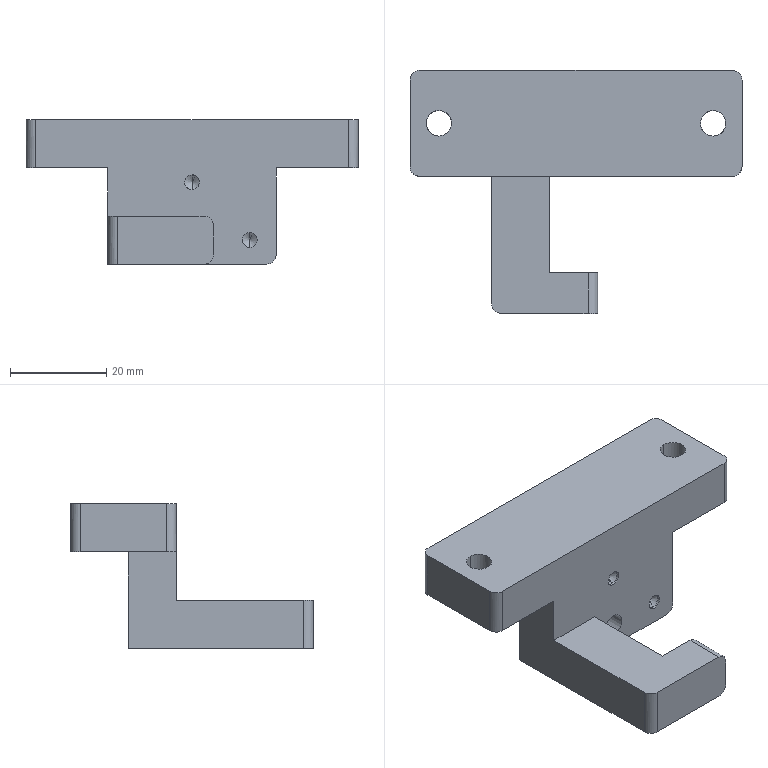NC program | NX | posted with a generic post | part box 69 x 50.5 x 30 mm
Lines 1 to 1585 of 2489:
N10 G17 G21 G94 G90
(FLOOR_WALL_COPY , TOOL : D80)
N12 T19 M6
N14 G54
N16 G17 G0 G90 X77.5 Y0. B0. C0. S6500 M3
N18 G43 Z30. H19
N20 Z7.
N22 G94 G1 Z4. F1500.
N24 X74.5
N26 X-74.5
N28 X-77.5
N30 Z7.
N32 G0 Z30.
N34 X77.5
N36 Z6.
N38 G1 Z3.
N40 X74.5
N42 X-74.5
N44 X-77.5
N46 Z6.
N48 G0 Z30.
N50 X77.5
N52 Z5.
N54 G1 Z2.
N56 X74.5
N58 X-74.5
N60 X-77.5
N62 Z5.
N64 G0 Z30.
N66 X77.5
N68 Z4.
N70 G1 Z1.
N72 X74.5
N74 X-74.5
N76 X-77.5
N78 Z4.
N80 G0 Z30.
N82 X77.5
N84 Z3.
N86 G1 Z0.
N88 X74.5
N90 X-74.5
N92 X-77.5
N94 Z3.
N96 G0 Z30.
N98 M5
(FLOOR_WALL_1_COPY_1 , TOOL : D10)
N100 T15 M6
N102 G54
N104 G17 G0 G90 X41. Y-12.807 B0. C0. S9500 M3
N106 G43 Z30. H15
N108 Z0.505
N110 G94 G1 Z-0.995 F3500.
N112 X40. Y-13.384
N114 G3 X39.5 Y-14.25 R1.
N116 G1 Y-23.479
N118 X39.403 Y-24.541
N120 X39.028 Y-25.845
N122 X38.378 Y-27.099
N124 X37.469 Y-28.219
N126 X36.349 Y-29.128
N128 X35.095 Y-29.778
N130 X33.791 Y-30.153
N132 X32.729 Y-30.25
N134 X-32.751
N136 X-33.878 Y-30.137
N138 X-35.185 Y-29.738
N140 X-36.392 Y-29.097
N142 X-37.468 Y-28.218
N144 X-38.347 Y-27.142
N146 X-38.988 Y-25.935
N148 X-39.387 Y-24.628
N150 X-39.5 Y-23.501
N152 Y-5.021
N154 X-39.403 Y-3.959
N156 X-39.028 Y-2.655
N158 X-38.378 Y-1.401
N160 X-37.469 Y-0.281
N162 X-36.349 Y0.628
N164 X-35.095 Y1.278
N166 X-33.791 Y1.653
N168 X-32.729 Y1.75
N170 X-22.6
N172 Y-18.35
N174 X-27.599 Y-23.25
N176 X-32.4
N178 X-32.491 Y-23.241
N180 X-32.492 Y-5.258
N182 X-32.408 Y-5.25
N184 X-29.6
N186 Y-18.35
N188 G3 X-27.599 Y-23.25 R7.
N190 G1 X-22.6 Y-18.35
N192 X22.6
N194 Y1.75
N196 X32.729
N198 X33.791 Y1.653
N200 X35.095 Y1.278
N202 X36.349 Y0.628
N204 X37.469 Y-0.281
N206 X38.378 Y-1.401
N208 X39.028 Y-2.655
N210 X39.403 Y-3.959
N212 X39.5 Y-5.021
N214 Y-14.25
N216 X32.5
N218 Y-23.158
N220 X32.492 Y-23.242
N222 X32.408 Y-23.25
N224 X27.599
N226 X22.6 Y-23.35
N228 X-22.6
N230 G2 X-23.016 Y-25.25 R5.
N232 G1 X23.016
N234 G2 X22.6 Y-23.35 R5.
N236 G1 X27.599 Y-23.25
N238 G3 X29.6 Y-18.35 R7.
N240 G1 Y-5.25
N242 X32.408
N244 X32.492 Y-5.258
N246 X32.5 Y-5.342
N248 Y-14.25
N250 G3 X33. Y-15.116 R1.
N252 G1 Z0.505
N254 G0 X41. Y-12.807 Z-0.49
N256 G1 Z-1.99
N258 X40. Y-13.384
N260 G3 X39.5 Y-14.25 R1.
N262 G1 Y-23.479
N264 X39.403 Y-24.541
N266 X39.028 Y-25.845
N268 X38.378 Y-27.099
N270 X37.469 Y-28.219
N272 X36.349 Y-29.128
N274 X35.095 Y-29.778
N276 X33.791 Y-30.153
N278 X32.729 Y-30.25
N280 X-32.751
N282 X-33.878 Y-30.137
N284 X-35.185 Y-29.738
N286 X-36.392 Y-29.097
N288 X-37.468 Y-28.218
N290 X-38.347 Y-27.142
N292 X-38.988 Y-25.935
N294 X-39.387 Y-24.628
N296 X-39.5 Y-23.501
N298 Y-5.021
N300 X-39.403 Y-3.959
N302 X-39.028 Y-2.655
N304 X-38.378 Y-1.401
N306 X-37.469 Y-0.281
N308 X-36.349 Y0.628
N310 X-35.095 Y1.278
N312 X-33.791 Y1.653
N314 X-32.729 Y1.75
N316 X-22.6
N318 Y-18.35
N320 X-27.599 Y-23.25
N322 X-32.4
N324 X-32.491 Y-23.241
N326 X-32.492 Y-5.258
N328 X-32.408 Y-5.25
N330 X-29.6
N332 Y-18.35
N334 G3 X-27.599 Y-23.25 R7.
N336 G1 X-22.6 Y-18.35
N338 X22.6
N340 Y1.75
N342 X32.729
N344 X33.791 Y1.653
N346 X35.095 Y1.278
N348 X36.349 Y0.628
N350 X37.469 Y-0.281
N352 X38.378 Y-1.401
N354 X39.028 Y-2.655
N356 X39.403 Y-3.959
N358 X39.5 Y-5.021
N360 Y-14.25
N362 X32.5
N364 Y-23.158
N366 X32.492 Y-23.242
N368 X32.408 Y-23.25
N370 X27.599
N372 X22.6 Y-23.35
N374 X-22.6
N376 G2 X-23.016 Y-25.25 R5.
N378 G1 X23.016
N380 G2 X22.6 Y-23.35 R5.
N382 G1 X27.599 Y-23.25
N384 G3 X29.6 Y-18.35 R7.
N386 G1 Y-5.25
N388 X32.408
N390 X32.492 Y-5.258
N392 X32.5 Y-5.342
N394 Y-14.25
N396 G3 X33. Y-15.116 R1.
N398 G1 Z-0.49
N400 G0 X41. Y-12.807 Z-1.485
N402 G1 Z-2.985
N404 X40. Y-13.384
N406 G3 X39.5 Y-14.25 R1.
N408 G1 Y-23.479
N410 X39.403 Y-24.541
N412 X39.028 Y-25.845
N414 X38.378 Y-27.099
N416 X37.469 Y-28.219
N418 X36.349 Y-29.128
N420 X35.095 Y-29.778
N422 X33.791 Y-30.153
N424 X32.729 Y-30.25
N426 X-32.751
N428 X-33.878 Y-30.137
N430 X-35.185 Y-29.738
N432 X-36.392 Y-29.097
N434 X-37.468 Y-28.218
N436 X-38.347 Y-27.142
N438 X-38.988 Y-25.935
N440 X-39.387 Y-24.628
N442 X-39.5 Y-23.501
N444 Y-5.021
N446 X-39.403 Y-3.959
N448 X-39.028 Y-2.655
N450 X-38.378 Y-1.401
N452 X-37.469 Y-0.281
N454 X-36.349 Y0.628
N456 X-35.095 Y1.278
N458 X-33.791 Y1.653
N460 X-32.729 Y1.75
N462 X-22.6
N464 Y-18.35
N466 X-27.599 Y-23.25
N468 X-32.4
N470 X-32.491 Y-23.241
N472 X-32.492 Y-5.258
N474 X-32.408 Y-5.25
N476 X-29.6
N478 Y-18.35
N480 G3 X-27.599 Y-23.25 R7.
N482 G1 X-22.6 Y-18.35
N484 X22.6
N486 Y1.75
N488 X32.729
N490 X33.791 Y1.653
N492 X35.095 Y1.278
N494 X36.349 Y0.628
N496 X37.469 Y-0.281
N498 X38.378 Y-1.401
N500 X39.028 Y-2.655
N502 X39.403 Y-3.959
N504 X39.5 Y-5.021
N506 Y-14.25
N508 X32.5
N510 Y-23.158
N512 X32.492 Y-23.242
N514 X32.408 Y-23.25
N516 X27.599
N518 X22.6 Y-23.35
N520 X-22.6
N522 G2 X-23.016 Y-25.25 R5.
N524 G1 X23.016
N526 G2 X22.6 Y-23.35 R5.
N528 G1 X27.599 Y-23.25
N530 G3 X29.6 Y-18.35 R7.
N532 G1 Y-5.25
N534 X32.408
N536 X32.492 Y-5.258
N538 X32.5 Y-5.342
N540 Y-14.25
N542 G3 X33. Y-15.116 R1.
N544 G1 Z-1.485
N546 G0 X41. Y-12.807 Z-2.48
N548 G1 Z-3.98
N550 X40. Y-13.384
N552 G3 X39.5 Y-14.25 R1.
N554 G1 Y-23.479
N556 X39.403 Y-24.541
N558 X39.028 Y-25.845
N560 X38.378 Y-27.099
N562 X37.469 Y-28.219
N564 X36.349 Y-29.128
N566 X35.095 Y-29.778
N568 X33.791 Y-30.153
N570 X32.729 Y-30.25
N572 X-32.751
N574 X-33.878 Y-30.137
N576 X-35.185 Y-29.738
N578 X-36.392 Y-29.097
N580 X-37.468 Y-28.218
N582 X-38.347 Y-27.142
N584 X-38.988 Y-25.935
N586 X-39.387 Y-24.628
N588 X-39.5 Y-23.501
N590 Y-5.021
N592 X-39.403 Y-3.959
N594 X-39.028 Y-2.655
N596 X-38.378 Y-1.401
N598 X-37.469 Y-0.281
N600 X-36.349 Y0.628
N602 X-35.095 Y1.278
N604 X-33.791 Y1.653
N606 X-32.729 Y1.75
N608 X-22.6
N610 Y-18.35
N612 X-27.599 Y-23.25
N614 X-32.4
N616 X-32.491 Y-23.241
N618 X-32.492 Y-5.258
N620 X-32.408 Y-5.25
N622 X-29.6
N624 Y-18.35
N626 G3 X-27.599 Y-23.25 R7.
N628 G1 X-22.6 Y-18.35
N630 X22.6
N632 Y1.75
N634 X32.729
N636 X33.791 Y1.653
N638 X35.095 Y1.278
N640 X36.349 Y0.628
N642 X37.469 Y-0.281
N644 X38.378 Y-1.401
N646 X39.028 Y-2.655
N648 X39.403 Y-3.959
N650 X39.5 Y-5.021
N652 Y-14.25
N654 X32.5
N656 Y-23.158
N658 X32.492 Y-23.242
N660 X32.408 Y-23.25
N662 X27.599
N664 X22.6 Y-23.35
N666 X-22.6
N668 G2 X-23.016 Y-25.25 R5.
N670 G1 X23.016
N672 G2 X22.6 Y-23.35 R5.
N674 G1 X27.599 Y-23.25
N676 G3 X29.6 Y-18.35 R7.
N678 G1 Y-5.25
N680 X32.408
N682 X32.492 Y-5.258
N684 X32.5 Y-5.342
N686 Y-14.25
N688 G3 X33. Y-15.116 R1.
N690 G1 Z-2.48
N692 G0 X41. Y-12.807 Z-3.475
N694 G1 Z-4.975
N696 X40. Y-13.384
N698 G3 X39.5 Y-14.25 R1.
N700 G1 Y-23.479
N702 X39.403 Y-24.541
N704 X39.028 Y-25.845
N706 X38.378 Y-27.099
N708 X37.469 Y-28.219
N710 X36.349 Y-29.128
N712 X35.095 Y-29.778
N714 X33.791 Y-30.153
N716 X32.729 Y-30.25
N718 X-32.751
N720 X-33.878 Y-30.137
N722 X-35.185 Y-29.738
N724 X-36.392 Y-29.097
N726 X-37.468 Y-28.218
N728 X-38.347 Y-27.142
N730 X-38.988 Y-25.935
N732 X-39.387 Y-24.628
N734 X-39.5 Y-23.501
N736 Y-5.021
N738 X-39.403 Y-3.959
N740 X-39.028 Y-2.655
N742 X-38.378 Y-1.401
N744 X-37.469 Y-0.281
N746 X-36.349 Y0.628
N748 X-35.095 Y1.278
N750 X-33.791 Y1.653
N752 X-32.729 Y1.75
N754 X-22.6
N756 Y-18.35
N758 X-27.599 Y-23.25
N760 X-32.4
N762 X-32.491 Y-23.241
N764 X-32.492 Y-5.258
N766 X-32.408 Y-5.25
N768 X-29.6
N770 Y-18.35
N772 G3 X-27.599 Y-23.25 R7.
N774 G1 X-22.6 Y-18.35
N776 X22.6
N778 Y1.75
N780 X32.729
N782 X33.791 Y1.653
N784 X35.095 Y1.278
N786 X36.349 Y0.628
N788 X37.469 Y-0.281
N790 X38.378 Y-1.401
N792 X39.028 Y-2.655
N794 X39.403 Y-3.959
N796 X39.5 Y-5.021
N798 Y-14.25
N800 X32.5
N802 Y-23.158
N804 X32.492 Y-23.242
N806 X32.408 Y-23.25
N808 X27.599
N810 X22.6 Y-23.35
N812 X-22.6
N814 G2 X-23.016 Y-25.25 R5.
N816 G1 X23.016
N818 G2 X22.6 Y-23.35 R5.
N820 G1 X27.599 Y-23.25
N822 G3 X29.6 Y-18.35 R7.
N824 G1 Y-5.25
N826 X32.408
N828 X32.492 Y-5.258
N830 X32.5 Y-5.342
N832 Y-14.25
N834 G3 X33. Y-15.116 R1.
N836 G1 Z-3.475
N838 G0 X41. Y-12.807 Z-4.47
N840 G1 Z-5.97
N842 X40. Y-13.384
N844 G3 X39.5 Y-14.25 R1.
N846 G1 Y-23.479
N848 X39.403 Y-24.541
N850 X39.028 Y-25.845
N852 X38.378 Y-27.099
N854 X37.469 Y-28.219
N856 X36.349 Y-29.128
N858 X35.095 Y-29.778
N860 X33.791 Y-30.153
N862 X32.729 Y-30.25
N864 X-32.751
N866 X-33.878 Y-30.137
N868 X-35.185 Y-29.738
N870 X-36.392 Y-29.097
N872 X-37.468 Y-28.218
N874 X-38.347 Y-27.142
N876 X-38.988 Y-25.935
N878 X-39.387 Y-24.628
N880 X-39.5 Y-23.501
N882 Y-5.021
N884 X-39.403 Y-3.959
N886 X-39.028 Y-2.655
N888 X-38.378 Y-1.401
N890 X-37.469 Y-0.281
N892 X-36.349 Y0.628
N894 X-35.095 Y1.278
N896 X-33.791 Y1.653
N898 X-32.729 Y1.75
N900 X-22.6
N902 Y-18.35
N904 X-27.599 Y-23.25
N906 X-32.4
N908 X-32.491 Y-23.241
N910 X-32.492 Y-5.258
N912 X-32.408 Y-5.25
N914 X-29.6
N916 Y-18.35
N918 G3 X-27.599 Y-23.25 R7.
N920 G1 X-22.6 Y-18.35
N922 X22.6
N924 Y1.75
N926 X32.729
N928 X33.791 Y1.653
N930 X35.095 Y1.278
N932 X36.349 Y0.628
N934 X37.469 Y-0.281
N936 X38.378 Y-1.401
N938 X39.028 Y-2.655
N940 X39.403 Y-3.959
N942 X39.5 Y-5.021
N944 Y-14.25
N946 X32.5
N948 Y-23.158
N950 X32.492 Y-23.242
N952 X32.408 Y-23.25
N954 X27.599
N956 X22.6 Y-23.35
N958 X-22.6
N960 G2 X-23.016 Y-25.25 R5.
N962 G1 X23.016
N964 G2 X22.6 Y-23.35 R5.
N966 G1 X27.599 Y-23.25
N968 G3 X29.6 Y-18.35 R7.
N970 G1 Y-5.25
N972 X32.408
N974 X32.492 Y-5.258
N976 X32.5 Y-5.342
N978 Y-14.25
N980 G3 X33. Y-15.116 R1.
N982 G1 Z-4.47
N984 G0 X41. Y-12.807 Z-5.465
N986 G1 Z-6.965
N988 X40. Y-13.384
N990 G3 X39.5 Y-14.25 R1.
N992 G1 Y-23.479
N994 X39.403 Y-24.541
N996 X39.028 Y-25.845
N998 X38.378 Y-27.099
N1000 X37.469 Y-28.219
N1002 X36.349 Y-29.128
N1004 X35.095 Y-29.778
N1006 X33.791 Y-30.153
N1008 X32.729 Y-30.25
N1010 X-32.751
N1012 X-33.878 Y-30.137
N1014 X-35.185 Y-29.738
N1016 X-36.392 Y-29.097
N1018 X-37.468 Y-28.218
N1020 X-38.347 Y-27.142
N1022 X-38.988 Y-25.935
N1024 X-39.387 Y-24.628
N1026 X-39.5 Y-23.501
N1028 Y-5.021
N1030 X-39.403 Y-3.959
N1032 X-39.028 Y-2.655
N1034 X-38.378 Y-1.401
N1036 X-37.469 Y-0.281
N1038 X-36.349 Y0.628
N1040 X-35.095 Y1.278
N1042 X-33.791 Y1.653
N1044 X-32.729 Y1.75
N1046 X-22.6
N1048 Y-18.35
N1050 X-27.599 Y-23.25
N1052 X-32.4
N1054 X-32.491 Y-23.241
N1056 X-32.492 Y-5.258
N1058 X-32.408 Y-5.25
N1060 X-29.6
N1062 Y-18.35
N1064 G3 X-27.599 Y-23.25 R7.
N1066 G1 X-22.6 Y-18.35
N1068 X22.6
N1070 Y1.75
N1072 X32.729
N1074 X33.791 Y1.653
N1076 X35.095 Y1.278
N1078 X36.349 Y0.628
N1080 X37.469 Y-0.281
N1082 X38.378 Y-1.401
N1084 X39.028 Y-2.655
N1086 X39.403 Y-3.959
N1088 X39.5 Y-5.021
N1090 Y-14.25
N1092 X32.5
N1094 Y-23.158
N1096 X32.492 Y-23.242
N1098 X32.408 Y-23.25
N1100 X27.599
N1102 X22.6 Y-23.35
N1104 X-22.6
N1106 G2 X-23.016 Y-25.25 R5.
N1108 G1 X23.016
N1110 G2 X22.6 Y-23.35 R5.
N1112 G1 X27.599 Y-23.25
N1114 G3 X29.6 Y-18.35 R7.
N1116 G1 Y-5.25
N1118 X32.408
N1120 X32.492 Y-5.258
N1122 X32.5 Y-5.342
N1124 Y-14.25
N1126 G3 X33. Y-15.116 R1.
N1128 G1 Z-5.465
N1130 G0 X41. Y-12.807 Z-6.46
N1132 G1 Z-7.96
N1134 X40. Y-13.384
N1136 G3 X39.5 Y-14.25 R1.
N1138 G1 Y-23.479
N1140 X39.403 Y-24.541
N1142 X39.028 Y-25.845
N1144 X38.378 Y-27.099
N1146 X37.469 Y-28.219
N1148 X36.349 Y-29.128
N1150 X35.095 Y-29.778
N1152 X33.791 Y-30.153
N1154 X32.729 Y-30.25
N1156 X-32.751
N1158 X-33.878 Y-30.137
N1160 X-35.185 Y-29.738
N1162 X-36.392 Y-29.097
N1164 X-37.468 Y-28.218
N1166 X-38.347 Y-27.142
N1168 X-38.988 Y-25.935
N1170 X-39.387 Y-24.628
N1172 X-39.5 Y-23.501
N1174 Y-5.021
N1176 X-39.403 Y-3.959
N1178 X-39.028 Y-2.655
N1180 X-38.378 Y-1.401
N1182 X-37.469 Y-0.281
N1184 X-36.349 Y0.628
N1186 X-35.095 Y1.278
N1188 X-33.791 Y1.653
N1190 X-32.729 Y1.75
N1192 X-22.6
N1194 Y-18.35
N1196 X-27.599 Y-23.25
N1198 X-32.4
N1200 X-32.491 Y-23.241
N1202 X-32.492 Y-5.258
N1204 X-32.408 Y-5.25
N1206 X-29.6
N1208 Y-18.35
N1210 G3 X-27.599 Y-23.25 R7.
N1212 G1 X-22.6 Y-18.35
N1214 X22.6
N1216 Y1.75
N1218 X32.729
N1220 X33.791 Y1.653
N1222 X35.095 Y1.278
N1224 X36.349 Y0.628
N1226 X37.469 Y-0.281
N1228 X38.378 Y-1.401
N1230 X39.028 Y-2.655
N1232 X39.403 Y-3.959
N1234 X39.5 Y-5.021
N1236 Y-14.25
N1238 X32.5
N1240 Y-23.158
N1242 X32.492 Y-23.242
N1244 X32.408 Y-23.25
N1246 X27.599
N1248 X22.6 Y-23.35
N1250 X-22.6
N1252 G2 X-23.016 Y-25.25 R5.
N1254 G1 X23.016
N1256 G2 X22.6 Y-23.35 R5.
N1258 G1 X27.599 Y-23.25
N1260 G3 X29.6 Y-18.35 R7.
N1262 G1 Y-5.25
N1264 X32.408
N1266 X32.492 Y-5.258
N1268 X32.5 Y-5.342
N1270 Y-14.25
N1272 G3 X33. Y-15.116 R1.
N1274 G1 Z-6.46
N1276 G0 X41. Y-12.807 Z-7.455
N1278 G1 Z-8.955
N1280 X40. Y-13.384
N1282 G3 X39.5 Y-14.25 R1.
N1284 G1 Y-23.479
N1286 X39.403 Y-24.541
N1288 X39.028 Y-25.845
N1290 X38.378 Y-27.099
N1292 X37.469 Y-28.219
N1294 X36.349 Y-29.128
N1296 X35.095 Y-29.778
N1298 X33.791 Y-30.153
N1300 X32.729 Y-30.25
N1302 X-32.751
N1304 X-33.878 Y-30.137
N1306 X-35.185 Y-29.738
N1308 X-36.392 Y-29.097
N1310 X-37.468 Y-28.218
N1312 X-38.347 Y-27.142
N1314 X-38.988 Y-25.935
N1316 X-39.387 Y-24.628
N1318 X-39.5 Y-23.501
N1320 Y-5.021
N1322 X-39.403 Y-3.959
N1324 X-39.028 Y-2.655
N1326 X-38.378 Y-1.401
N1328 X-37.469 Y-0.281
N1330 X-36.349 Y0.628
N1332 X-35.095 Y1.278
N1334 X-33.791 Y1.653
N1336 X-32.729 Y1.75
N1338 X-22.6
N1340 Y-18.35
N1342 X-27.599 Y-23.25
N1344 X-32.4
N1346 X-32.491 Y-23.241
N1348 X-32.492 Y-5.258
N1350 X-32.408 Y-5.25
N1352 X-29.6
N1354 Y-18.35
N1356 G3 X-27.599 Y-23.25 R7.
N1358 G1 X-22.6 Y-18.35
N1360 X22.6
N1362 Y1.75
N1364 X32.729
N1366 X33.791 Y1.653
N1368 X35.095 Y1.278
N1370 X36.349 Y0.628
N1372 X37.469 Y-0.281
N1374 X38.378 Y-1.401
N1376 X39.028 Y-2.655
N1378 X39.403 Y-3.959
N1380 X39.5 Y-5.021
N1382 Y-14.25
N1384 X32.5
N1386 Y-23.158
N1388 X32.492 Y-23.242
N1390 X32.408 Y-23.25
N1392 X27.599
N1394 X22.6 Y-23.35
N1396 X-22.6
N1398 G2 X-23.016 Y-25.25 R5.
N1400 G1 X23.016
N1402 G2 X22.6 Y-23.35 R5.
N1404 G1 X27.599 Y-23.25
N1406 G3 X29.6 Y-18.35 R7.
N1408 G1 Y-5.25
N1410 X32.408
N1412 X32.492 Y-5.258
N1414 X32.5 Y-5.342
N1416 Y-14.25
N1418 G3 X33. Y-15.116 R1.
N1420 G1 Z-7.455
N1422 G0 X41. Y-12.807 Z-8.45
N1424 G1 Z-9.95
N1426 X40. Y-13.384
N1428 G3 X39.5 Y-14.25 R1.
N1430 G1 Y-23.479
N1432 X39.403 Y-24.541
N1434 X39.028 Y-25.845
N1436 X38.378 Y-27.099
N1438 X37.469 Y-28.219
N1440 X36.349 Y-29.128
N1442 X35.095 Y-29.778
N1444 X33.791 Y-30.153
N1446 X32.729 Y-30.25
N1448 X-32.751
N1450 X-33.878 Y-30.137
N1452 X-35.185 Y-29.738
N1454 X-36.392 Y-29.097
N1456 X-37.468 Y-28.218
N1458 X-38.347 Y-27.142
N1460 X-38.988 Y-25.935
N1462 X-39.387 Y-24.628
N1464 X-39.5 Y-23.501
N1466 Y-5.021
N1468 X-39.403 Y-3.959
N1470 X-39.028 Y-2.655
N1472 X-38.378 Y-1.401
N1474 X-37.469 Y-0.281
N1476 X-36.349 Y0.628
N1478 X-35.095 Y1.278
N1480 X-33.791 Y1.653
N1482 X-32.729 Y1.75
N1484 X-22.6
N1486 Y-18.35
N1488 X-27.599 Y-23.25
N1490 X-32.4
N1492 X-32.491 Y-23.241
N1494 X-32.492 Y-5.258
N1496 X-32.408 Y-5.25
N1498 X-29.6
N1500 Y-18.35
N1502 G3 X-27.599 Y-23.25 R7.
N1504 G1 X-22.6 Y-18.35
N1506 X22.6
N1508 Y1.75
N1510 X32.729
N1512 X33.791 Y1.653
N1514 X35.095 Y1.278
N1516 X36.349 Y0.628
N1518 X37.469 Y-0.281
N1520 X38.378 Y-1.401
N1522 X39.028 Y-2.655
N1524 X39.403 Y-3.959
N1526 X39.5 Y-5.021
N1528 Y-14.25
N1530 X32.5
N1532 Y-23.158
N1534 X32.492 Y-23.242
N1536 X32.408 Y-23.25
N1538 X27.599
N1540 X22.6 Y-23.35
N1542 X-22.6
N1544 G2 X-23.016 Y-25.25 R5.
N1546 G1 X23.016
N1548 G2 X22.6 Y-23.35 R5.
N1550 G1 X27.599 Y-23.25
N1552 G3 X29.6 Y-18.35 R7.
N1554 G1 Y-5.25
N1556 X32.408
N1558 X32.492 Y-5.258
N1560 X32.5 Y-5.342
N1562 Y-14.25
N1564 G3 X33. Y-15.116 R1.
N1566 G1 Z-8.45
N1568 G0 X41. Y-12.807 Z-9.445
N1570 G1 Z-10.945
N1572 X40. Y-13.384
N1574 G3 X39.5 Y-14.25 R1.
N1576 G1 Y-23.479
N1578 X39.403 Y-24.541
N1580 X39.028 Y-25.845
N1582 X38.378 Y-27.099
N1584 X37.469 Y-28.219
N1586 X36.349 Y-29.128
N1588 X35.095 Y-29.778
N1590 X33.791 Y-30.153
N1592 X32.729 Y-30.25
N1594 X-32.751
N1596 X-33.878 Y-30.137
N1598 X-35.185 Y-29.738
N1600 X-36.392 Y-29.097
N1602 X-37.468 Y-28.218
N1604 X-38.347 Y-27.142
N1606 X-38.988 Y-25.935
N1608 X-39.387 Y-24.628
N1610 X-39.5 Y-23.501
N1612 Y-5.021
N1614 X-39.403 Y-3.959
N1616 X-39.028 Y-2.655
N1618 X-38.378 Y-1.401
N1620 X-37.469 Y-0.281
N1622 X-36.349 Y0.628
N1624 X-35.095 Y1.278
N1626 X-33.791 Y1.653
N1628 X-32.729 Y1.75
N1630 X-22.6
N1632 Y-18.35
N1634 X-27.599 Y-23.25
N1636 X-32.4
N1638 X-32.491 Y-23.241
N1640 X-32.492 Y-5.258
N1642 X-32.408 Y-5.25
N1644 X-29.6
N1646 Y-18.35
N1648 G3 X-27.599 Y-23.25 R7.
N1650 G1 X-22.6 Y-18.35
N1652 X22.6
N1654 Y1.75
N1656 X32.729
N1658 X33.791 Y1.653
N1660 X35.095 Y1.278
N1662 X36.349 Y0.628
N1664 X37.469 Y-0.281
N1666 X38.378 Y-1.401
N1668 X39.028 Y-2.655
N1670 X39.403 Y-3.959
N1672 X39.5 Y-5.021
N1674 Y-14.25
N1676 X32.5
N1678 Y-23.158
N1680 X32.492 Y-23.242
N1682 X32.408 Y-23.25
N1684 X27.599
N1686 X22.6 Y-23.35
N1688 X-22.6
N1690 G2 X-23.016 Y-25.25 R5.
N1692 G1 X23.016
N1694 G2 X22.6 Y-23.35 R5.
N1696 G1 X27.599 Y-23.25
N1698 G3 X29.6 Y-18.35 R7.
N1700 G1 Y-5.25
N1702 X32.408
N1704 X32.492 Y-5.258
N1706 X32.5 Y-5.342
N1708 Y-14.25
N1710 G3 X33. Y-15.116 R1.
N1712 G1 Z-9.445
N1714 G0 X41. Y-12.807 Z-10.44
N1716 G1 Z-11.94
N1718 X40. Y-13.384
N1720 G3 X39.5 Y-14.25 R1.
N1722 G1 Y-23.479
N1724 X39.403 Y-24.541
N1726 X39.028 Y-25.845
N1728 X38.378 Y-27.099
N1730 X37.469 Y-28.219
N1732 X36.349 Y-29.128
N1734 X35.095 Y-29.778
N1736 X33.791 Y-30.153
N1738 X32.729 Y-30.25
N1740 X-32.751
N1742 X-33.878 Y-30.137
N1744 X-35.185 Y-29.738
N1746 X-36.392 Y-29.097
N1748 X-37.468 Y-28.218
N1750 X-38.347 Y-27.142
N1752 X-38.988 Y-25.935
N1754 X-39.387 Y-24.628
N1756 X-39.5 Y-23.501
N1758 Y-5.021
N1760 X-39.403 Y-3.959
N1762 X-39.028 Y-2.655
N1764 X-38.378 Y-1.401
N1766 X-37.469 Y-0.281
N1768 X-36.349 Y0.628
N1770 X-35.095 Y1.278
N1772 X-33.791 Y1.653
N1774 X-32.729 Y1.75
N1776 X-22.6
N1778 Y-18.35
N1780 X-27.599 Y-23.25
N1782 X-32.4
N1784 X-32.491 Y-23.241
N1786 X-32.492 Y-5.258
N1788 X-32.408 Y-5.25
N1790 X-29.6
N1792 Y-18.35
N1794 G3 X-27.599 Y-23.25 R7.
N1796 G1 X-22.6 Y-18.35
N1798 X22.6
N1800 Y1.75
N1802 X32.729
N1804 X33.791 Y1.653
N1806 X35.095 Y1.278
N1808 X36.349 Y0.628
N1810 X37.469 Y-0.281
N1812 X38.378 Y-1.401
N1814 X39.028 Y-2.655
N1816 X39.403 Y-3.959
N1818 X39.5 Y-5.021
N1820 Y-14.25
N1822 X32.5
N1824 Y-23.158
N1826 X32.492 Y-23.242
N1828 X32.408 Y-23.25
N1830 X27.599
N1832 X22.6 Y-23.35
N1834 X-22.6
N1836 G2 X-23.016 Y-25.25 R5.
N1838 G1 X23.016
N1840 G2 X22.6 Y-23.35 R5.
N1842 G1 X27.599 Y-23.25
N1844 G3 X29.6 Y-18.35 R7.
N1846 G1 Y-5.25
N1848 X32.408
N1850 X32.492 Y-5.258
N1852 X32.5 Y-5.342
N1854 Y-14.25
N1856 G3 X33. Y-15.116 R1.
N1858 G1 Z-10.44
N1860 G0 X41. Y-12.807 Z-11.435
N1862 G1 Z-12.935
N1864 X40. Y-13.384
N1866 G3 X39.5 Y-14.25 R1.
N1868 G1 Y-23.479
N1870 X39.403 Y-24.541
N1872 X39.028 Y-25.845
N1874 X38.378 Y-27.099
N1876 X37.469 Y-28.219
N1878 X36.349 Y-29.128
N1880 X35.095 Y-29.778
N1882 X33.791 Y-30.153
N1884 X32.729 Y-30.25
N1886 X-32.751
N1888 X-33.878 Y-30.137
N1890 X-35.185 Y-29.738
N1892 X-36.392 Y-29.097
N1894 X-37.468 Y-28.218
N1896 X-38.347 Y-27.142
N1898 X-38.988 Y-25.935
N1900 X-39.387 Y-24.628
N1902 X-39.5 Y-23.501
N1904 Y-5.021
N1906 X-39.403 Y-3.959
N1908 X-39.028 Y-2.655
N1910 X-38.378 Y-1.401
N1912 X-37.469 Y-0.281
N1914 X-36.349 Y0.628
N1916 X-35.095 Y1.278
N1918 X-33.791 Y1.653
N1920 X-32.729 Y1.75
N1922 X-22.6
N1924 Y-18.35
N1926 X-27.599 Y-23.25
N1928 X-32.4
N1930 X-32.491 Y-23.241
N1932 X-32.492 Y-5.258
N1934 X-32.408 Y-5.25
N1936 X-29.6
N1938 Y-18.35
N1940 G3 X-27.599 Y-23.25 R7.
N1942 G1 X-22.6 Y-18.35
N1944 X22.6
N1946 Y1.75
N1948 X32.729
N1950 X33.791 Y1.653
N1952 X35.095 Y1.278
N1954 X36.349 Y0.628
N1956 X37.469 Y-0.281
N1958 X38.378 Y-1.401
N1960 X39.028 Y-2.655
N1962 X39.403 Y-3.959
N1964 X39.5 Y-5.021
N1966 Y-14.25
N1968 X32.5
N1970 Y-23.158
N1972 X32.492 Y-23.242
N1974 X32.408 Y-23.25
N1976 X27.599
N1978 X22.6 Y-23.35
N1980 X-22.6
N1982 G2 X-23.016 Y-25.25 R5.
N1984 G1 X23.016
N1986 G2 X22.6 Y-23.35 R5.
N1988 G1 X27.599 Y-23.25
N1990 G3 X29.6 Y-18.35 R7.
N1992 G1 Y-5.25
N1994 X32.408
N1996 X32.492 Y-5.258
N1998 X32.5 Y-5.342
N2000 Y-14.25
N2002 G3 X33. Y-15.116 R1.
N2004 G1 Z-11.435
N2006 G0 X41. Y-12.807 Z-12.43
N2008 G1 Z-13.93
N2010 X40. Y-13.384
N2012 G3 X39.5 Y-14.25 R1.
N2014 G1 Y-23.479
N2016 X39.403 Y-24.541
N2018 X39.028 Y-25.845
N2020 X38.378 Y-27.099
N2022 X37.469 Y-28.219
N2024 X36.349 Y-29.128
N2026 X35.095 Y-29.778
N2028 X33.791 Y-30.153
N2030 X32.729 Y-30.25
N2032 X-32.751
N2034 X-33.878 Y-30.137
N2036 X-35.185 Y-29.738
N2038 X-36.392 Y-29.097
N2040 X-37.468 Y-28.218
N2042 X-38.347 Y-27.142
N2044 X-38.988 Y-25.935
N2046 X-39.387 Y-24.628
N2048 X-39.5 Y-23.501
N2050 Y-5.021
N2052 X-39.403 Y-3.959
N2054 X-39.028 Y-2.655
N2056 X-38.378 Y-1.401
N2058 X-37.469 Y-0.281
N2060 X-36.349 Y0.628
N2062 X-35.095 Y1.278
N2064 X-33.791 Y1.653
N2066 X-32.729 Y1.75
N2068 X-22.6
N2070 Y-18.35
N2072 X-27.599 Y-23.25
N2074 X-32.4
N2076 X-32.491 Y-23.241
N2078 X-32.492 Y-5.258
N2080 X-32.408 Y-5.25
N2082 X-29.6
N2084 Y-18.35
N2086 G3 X-27.599 Y-23.25 R7.
N2088 G1 X-22.6 Y-18.35
N2090 X22.6
N2092 Y1.75
N2094 X32.729
N2096 X33.791 Y1.653
N2098 X35.095 Y1.278
N2100 X36.349 Y0.628
N2102 X37.469 Y-0.281
N2104 X38.378 Y-1.401
N2106 X39.028 Y-2.655
N2108 X39.403 Y-3.959
N2110 X39.5 Y-5.021
N2112 Y-14.25
N2114 X32.5
N2116 Y-23.158
N2118 X32.492 Y-23.242
N2120 X32.408 Y-23.25
N2122 X27.599
N2124 X22.6 Y-23.35
N2126 X-22.6
N2128 G2 X-23.016 Y-25.25 R5.
N2130 G1 X23.016
N2132 G2 X22.6 Y-23.35 R5.
N2134 G1 X27.599 Y-23.25
N2136 G3 X29.6 Y-18.35 R7.
N2138 G1 Y-5.25
N2140 X32.408
N2142 X32.492 Y-5.258
N2144 X32.5 Y-5.342
N2146 Y-14.25
N2148 G3 X33. Y-15.116 R1.
N2150 G1 Z-12.43
N2152 G0 X41. Y-12.807 Z-13.425
N2154 G1 Z-14.925
N2156 X40. Y-13.384
N2158 G3 X39.5 Y-14.25 R1.
N2160 G1 Y-23.479
N2162 X39.403 Y-24.541
N2164 X39.028 Y-25.845
N2166 X38.378 Y-27.099
N2168 X37.469 Y-28.219
N2170 X36.349 Y-29.128
N2172 X35.095 Y-29.778
N2174 X33.791 Y-30.153
N2176 X32.729 Y-30.25
N2178 X-32.751
N2180 X-33.878 Y-30.137
N2182 X-35.185 Y-29.738
N2184 X-36.392 Y-29.097
N2186 X-37.468 Y-28.218
N2188 X-38.347 Y-27.142
N2190 X-38.988 Y-25.935
N2192 X-39.387 Y-24.628
N2194 X-39.5 Y-23.501
N2196 Y-5.021
N2198 X-39.403 Y-3.959
N2200 X-39.028 Y-2.655
N2202 X-38.378 Y-1.401
N2204 X-37.469 Y-0.281
N2206 X-36.349 Y0.628
N2208 X-35.095 Y1.278
N2210 X-33.791 Y1.653
N2212 X-32.729 Y1.75
N2214 X-22.6
N2216 Y-18.35
N2218 X-27.599 Y-23.25
N2220 X-32.4
N2222 X-32.491 Y-23.241
N2224 X-32.492 Y-5.258
N2226 X-32.408 Y-5.25
N2228 X-29.6
N2230 Y-18.35
N2232 G3 X-27.599 Y-23.25 R7.
N2234 G1 X-22.6 Y-18.35
N2236 X22.6
N2238 Y1.75
N2240 X32.729
N2242 X33.791 Y1.653
N2244 X35.095 Y1.278
N2246 X36.349 Y0.628
N2248 X37.469 Y-0.281
N2250 X38.378 Y-1.401
N2252 X39.028 Y-2.655
N2254 X39.403 Y-3.959
N2256 X39.5 Y-5.021
N2258 Y-14.25
N2260 X32.5
N2262 Y-23.158
N2264 X32.492 Y-23.242
N2266 X32.408 Y-23.25
N2268 X27.599
N2270 X22.6 Y-23.35
N2272 X-22.6
N2274 G2 X-23.016 Y-25.25 R5.
N2276 G1 X23.016
N2278 G2 X22.6 Y-23.35 R5.
N2280 G1 X27.599 Y-23.25
N2282 G3 X29.6 Y-18.35 R7.
N2284 G1 Y-5.25
N2286 X32.408
N2288 X32.492 Y-5.258
N2290 X32.5 Y-5.342
N2292 Y-14.25
N2294 G3 X33. Y-15.116 R1.
N2296 G1 Z-13.425
N2298 G0 X41. Y-12.807 Z-14.42
N2300 G1 Z-15.92
N2302 X40. Y-13.384
N2304 G3 X39.5 Y-14.25 R1.
N2306 G1 Y-23.479
N2308 X39.403 Y-24.541
N2310 X39.028 Y-25.845
N2312 X38.378 Y-27.099
N2314 X37.469 Y-28.219
N2316 X36.349 Y-29.128
N2318 X35.095 Y-29.778
N2320 X33.791 Y-30.153
N2322 X32.729 Y-30.25
N2324 X-32.751
N2326 X-33.878 Y-30.137
N2328 X-35.185 Y-29.738
N2330 X-36.392 Y-29.097
N2332 X-37.468 Y-28.218
N2334 X-38.347 Y-27.142
N2336 X-38.988 Y-25.935
N2338 X-39.387 Y-24.628
N2340 X-39.5 Y-23.501
N2342 Y-5.021
N2344 X-39.403 Y-3.959
N2346 X-39.028 Y-2.655
N2348 X-38.378 Y-1.401
N2350 X-37.469 Y-0.281
N2352 X-36.349 Y0.628
N2354 X-35.095 Y1.278
N2356 X-33.791 Y1.653
N2358 X-32.729 Y1.75
N2360 X-22.6
N2362 Y-18.35
N2364 X-27.599 Y-23.25
N2366 X-32.4
N2368 X-32.491 Y-23.241
N2370 X-32.492 Y-5.258
N2372 X-32.408 Y-5.25
N2374 X-29.6
N2376 Y-18.35
N2378 G3 X-27.599 Y-23.25 R7.
N2380 G1 X-22.6 Y-18.35
N2382 X22.6
N2384 Y1.75
N2386 X32.729
N2388 X33.791 Y1.653
N2390 X35.095 Y1.278
N2392 X36.349 Y0.628
N2394 X37.469 Y-0.281
N2396 X38.378 Y-1.401
N2398 X39.028 Y-2.655
N2400 X39.403 Y-3.959
N2402 X39.5 Y-5.021
N2404 Y-14.25
N2406 X32.5
N2408 Y-23.158
N2410 X32.492 Y-23.242
N2412 X32.408 Y-23.25
N2414 X27.599
N2416 X22.6 Y-23.35
N2418 X-22.6
N2420 G2 X-23.016 Y-25.25 R5.
N2422 G1 X23.016
N2424 G2 X22.6 Y-23.35 R5.
N2426 G1 X27.599 Y-23.25
N2428 G3 X29.6 Y-18.35 R7.
N2430 G1 Y-5.25
N2432 X32.408
N2434 X32.492 Y-5.258
N2436 X32.5 Y-5.342
N2438 Y-14.25
N2440 G3 X33. Y-15.116 R1.
N2442 G1 Z-14.42
N2444 G0 X41. Y-12.807 Z-15.415
N2446 G1 Z-16.915
N2448 X40. Y-13.384
N2450 G3 X39.5 Y-14.25 R1.
N2452 G1 Y-23.479
N2454 X39.403 Y-24.541
N2456 X39.028 Y-25.845
N2458 X38.378 Y-27.099
N2460 X37.469 Y-28.219
N2462 X36.349 Y-29.128
N2464 X35.095 Y-29.778
N2466 X33.791 Y-30.153
N2468 X32.729 Y-30.25
N2470 X-32.751
N2472 X-33.878 Y-30.137
N2474 X-35.185 Y-29.738
N2476 X-36.392 Y-29.097
N2478 X-37.468 Y-28.218
N2480 X-38.347 Y-27.142
N2482 X-38.988 Y-25.935
N2484 X-39.387 Y-24.628
N2486 X-39.5 Y-23.501
N2488 Y-5.021
N2490 X-39.403 Y-3.959
N2492 X-39.028 Y-2.655
N2494 X-38.378 Y-1.401
N2496 X-37.469 Y-0.281
N2498 X-36.349 Y0.628
N2500 X-35.095 Y1.278
N2502 X-33.791 Y1.653
N2504 X-32.729 Y1.75
N2506 X-22.6
N2508 Y-18.35
N2510 X-27.599 Y-23.25
N2512 X-32.4
N2514 X-32.491 Y-23.241
N2516 X-32.492 Y-5.258
N2518 X-32.408 Y-5.25
N2520 X-29.6
N2522 Y-18.35
N2524 G3 X-27.599 Y-23.25 R7.
N2526 G1 X-22.6 Y-18.35
N2528 X22.6
N2530 Y1.75
N2532 X32.729
N2534 X33.791 Y1.653
N2536 X35.095 Y1.278
N2538 X36.349 Y0.628
N2540 X37.469 Y-0.281
N2542 X38.378 Y-1.401
N2544 X39.028 Y-2.655
N2546 X39.403 Y-3.959
N2548 X39.5 Y-5.021
N2550 Y-14.25
N2552 X32.5
N2554 Y-23.158
N2556 X32.492 Y-23.242
N2558 X32.408 Y-23.25
N2560 X27.599
N2562 X22.6 Y-23.35
N2564 X-22.6
N2566 G2 X-23.016 Y-25.25 R5.
N2568 G1 X23.016
N2570 G2 X22.6 Y-23.35 R5.
N2572 G1 X27.599 Y-23.25
N2574 G3 X29.6 Y-18.35 R7.
N2576 G1 Y-5.25
N2578 X32.408
N2580 X32.492 Y-5.258
N2582 X32.5 Y-5.342
N2584 Y-14.25
N2586 G3 X33. Y-15.116 R1.
N2588 G1 Z-15.415
N2590 G0 X41. Y-12.807 Z-16.41
N2592 G1 Z-17.91
N2594 X40. Y-13.384
N2596 G3 X39.5 Y-14.25 R1.
N2598 G1 Y-23.479
N2600 X39.403 Y-24.541
N2602 X39.028 Y-25.845
N2604 X38.378 Y-27.099
N2606 X37.469 Y-28.219
N2608 X36.349 Y-29.128
N2610 X35.095 Y-29.778
N2612 X33.791 Y-30.153
N2614 X32.729 Y-30.25
N2616 X-32.751
N2618 X-33.878 Y-30.137
N2620 X-35.185 Y-29.738
N2622 X-36.392 Y-29.097
N2624 X-37.468 Y-28.218
N2626 X-38.347 Y-27.142
N2628 X-38.988 Y-25.935
N2630 X-39.387 Y-24.628
N2632 X-39.5 Y-23.501
N2634 Y-5.021
N2636 X-39.403 Y-3.959
N2638 X-39.028 Y-2.655
N2640 X-38.378 Y-1.401
N2642 X-37.469 Y-0.281
N2644 X-36.349 Y0.628
N2646 X-35.095 Y1.278
N2648 X-33.791 Y1.653
N2650 X-32.729 Y1.75
N2652 X-22.6
N2654 Y-18.35
N2656 X-27.599 Y-23.25
N2658 X-32.4
N2660 X-32.491 Y-23.241
N2662 X-32.492 Y-5.258
N2664 X-32.408 Y-5.25
N2666 X-29.6
N2668 Y-18.35
N2670 G3 X-27.599 Y-23.25 R7.
N2672 G1 X-22.6 Y-18.35
N2674 X22.6
N2676 Y1.75
N2678 X32.729
N2680 X33.791 Y1.653
N2682 X35.095 Y1.278
N2684 X36.349 Y0.628
N2686 X37.469 Y-0.281
N2688 X38.378 Y-1.401
N2690 X39.028 Y-2.655
N2692 X39.403 Y-3.959
N2694 X39.5 Y-5.021
N2696 Y-14.25
N2698 X32.5
N2700 Y-23.158
N2702 X32.492 Y-23.242
N2704 X32.408 Y-23.25
N2706 X27.599
N2708 X22.6 Y-23.35
N2710 X-22.6
N2712 G2 X-23.016 Y-25.25 R5.
N2714 G1 X23.016
N2716 G2 X22.6 Y-23.35 R5.
N2718 G1 X27.599 Y-23.25
N2720 G3 X29.6 Y-18.35 R7.
N2722 G1 Y-5.25
N2724 X32.408
N2726 X32.492 Y-5.258
N2728 X32.5 Y-5.342
N2730 Y-14.25
N2732 G3 X33. Y-15.116 R1.
N2734 G1 Z-16.41
N2736 G0 X41. Y-12.807 Z-17.405
N2738 G1 Z-18.905
N2740 X40. Y-13.384
N2742 G3 X39.5 Y-14.25 R1.
N2744 G1 Y-23.479
N2746 X39.403 Y-24.541
N2748 X39.028 Y-25.845
N2750 X38.378 Y-27.099
N2752 X37.469 Y-28.219
N2754 X36.349 Y-29.128
N2756 X35.095 Y-29.778
N2758 X33.791 Y-30.153
N2760 X32.729 Y-30.25
N2762 X-32.751
N2764 X-33.878 Y-30.137
N2766 X-35.185 Y-29.738
N2768 X-36.392 Y-29.097
N2770 X-37.468 Y-28.218
N2772 X-38.347 Y-27.142
N2774 X-38.988 Y-25.935
N2776 X-39.387 Y-24.628
N2778 X-39.5 Y-23.501
N2780 Y-5.021
N2782 X-39.403 Y-3.959
N2784 X-39.028 Y-2.655
N2786 X-38.378 Y-1.401
N2788 X-37.469 Y-0.281
N2790 X-36.349 Y0.628
N2792 X-35.095 Y1.278
N2794 X-33.791 Y1.653
N2796 X-32.729 Y1.75
N2798 X-22.6
N2800 Y-18.35
N2802 X-27.599 Y-23.25
N2804 X-32.4
N2806 X-32.491 Y-23.241
N2808 X-32.492 Y-5.258
N2810 X-32.408 Y-5.25
N2812 X-29.6
N2814 Y-18.35
N2816 G3 X-27.599 Y-23.25 R7.
N2818 G1 X-22.6 Y-18.35
N2820 X22.6
N2822 Y1.75
N2824 X32.729
N2826 X33.791 Y1.653
N2828 X35.095 Y1.278
N2830 X36.349 Y0.628
N2832 X37.469 Y-0.281
N2834 X38.378 Y-1.401
N2836 X39.028 Y-2.655
N2838 X39.403 Y-3.959
N2840 X39.5 Y-5.021
N2842 Y-14.25
N2844 X32.5
N2846 Y-23.158
N2848 X32.492 Y-23.242
N2850 X32.408 Y-23.25
N2852 X27.599
N2854 X22.6 Y-23.35
N2856 X-22.6
N2858 G2 X-23.016 Y-25.25 R5.
N2860 G1 X23.016
N2862 G2 X22.6 Y-23.35 R5.
N2864 G1 X27.599 Y-23.25
N2866 G3 X29.6 Y-18.35 R7.
N2868 G1 Y-5.25
N2870 X32.408
N2872 X32.492 Y-5.258
N2874 X32.5 Y-5.342
N2876 Y-14.25
N2878 G3 X33. Y-15.116 R1.
N2880 G1 Z-17.405
N2882 G0 X41. Y-12.807 Z-18.4
N2884 G1 Z-19.9
N2886 X40. Y-13.384
N2888 G3 X39.5 Y-14.25 R1.
N2890 G1 Y-23.479
N2892 X39.403 Y-24.541
N2894 X39.028 Y-25.845
N2896 X38.378 Y-27.099
N2898 X37.469 Y-28.219
N2900 X36.349 Y-29.128
N2902 X35.095 Y-29.778
N2904 X33.791 Y-30.153
N2906 X32.729 Y-30.25
N2908 X-32.751
N2910 X-33.878 Y-30.137
N2912 X-35.185 Y-29.738
N2914 X-36.392 Y-29.097
N2916 X-37.468 Y-28.218
N2918 X-38.347 Y-27.142
N2920 X-38.988 Y-25.935
N2922 X-39.387 Y-24.628
N2924 X-39.5 Y-23.501
N2926 Y-5.021
N2928 X-39.403 Y-3.959
N2930 X-39.028 Y-2.655
N2932 X-38.378 Y-1.401
N2934 X-37.469 Y-0.281
N2936 X-36.349 Y0.628
N2938 X-35.095 Y1.278
N2940 X-33.791 Y1.653
N2942 X-32.729 Y1.75
N2944 X-22.6
N2946 Y-18.35
N2948 X-27.599 Y-23.25
N2950 X-32.4
N2952 X-32.491 Y-23.241
N2954 X-32.492 Y-5.258
N2956 X-32.408 Y-5.25
N2958 X-29.6
N2960 Y-18.35
N2962 G3 X-27.599 Y-23.25 R7.
N2964 G1 X-22.6 Y-18.35
N2966 X22.6
N2968 Y1.75
N2970 X32.729
N2972 X33.791 Y1.653
N2974 X35.095 Y1.278
N2976 X36.349 Y0.628
N2978 X37.469 Y-0.281
N2980 X38.378 Y-1.401
N2982 X39.028 Y-2.655
N2984 X39.403 Y-3.959
N2986 X39.5 Y-5.021
N2988 Y-14.25
N2990 X32.5
N2992 Y-23.158
N2994 X32.492 Y-23.242
N2996 X32.408 Y-23.25
N2998 X27.599
N3000 X22.6 Y-23.35
N3002 X-22.6
N3004 G2 X-23.016 Y-25.25 R5.
N3006 G1 X23.016
N3008 G2 X22.6 Y-23.35 R5.
N3010 G1 X27.599 Y-23.25
N3012 G3 X29.6 Y-18.35 R7.
N3014 G1 Y-5.25
N3016 X32.408
N3018 X32.492 Y-5.258
N3020 X32.5 Y-5.342
N3022 Y-14.25
N3024 G3 X33. Y-15.116 R1.
N3026 G1 Z-18.4
N3028 G0 Z30.
N3030 M5
(FLOOR_WALL_1_COPY_COPY_1_COPY , TOOL : D10JING)
N3032 T14 M6
N3034 G54
N3036 G17 G0 G90 X34.098 Y-31.621 B0. C0. S9500 M3
N3038 G43 Z30. H14
N3040 Z-18.5
N3042 G94 G1 Z-20. F1200.
N3044 X33.595 Y-30.75
N3046 G3 X32.729 Y-30.25 R1.
N3048 G1 X-32.751
N3050 X-33.878 Y-30.137
N3052 X-35.185 Y-29.738
N3054 X-36.392 Y-29.097
N3056 X-37.468 Y-28.218
N3058 X-38.347 Y-27.142
N3060 X-38.988 Y-25.935
N3062 X-39.075 Y-25.65
N3064 X39.084
N3066 X39.403 Y-24.541
N3068 X39.5 Y-23.479
N3070 Y-21.05
N3072 X-39.5
N3074 Y-16.45
N3076 X-23.
N3078 Y-11.85
N3080 X-39.5
N3082 Y-7.25
N3084 X-23.
N3086 Y-2.65
N3088 X-39.025
N3090 G3 X-39.891 Y-3.15 R1.
N3092 G1 X-41. Y-5.071
N3094 Z-18.5
N3096 G0 X-23. Y-16.45
N3098 G1 Z-20.
N3100 Y-18.25
N3102 G3 X-22.5 Y-18.75 R0.5
N3104 G1 X22.5
N3106 G3 X23. Y-18.25 R0.5
N3108 G1 Y-16.45
N3110 X39.5
N3112 Y-11.85
N3114 X23.
N3116 Y-7.25
N3118 X39.5
N3120 Y-5.021
N3122 X39.403 Y-3.959
N3124 X39.028 Y-2.655
N3126 X39.025 Y-2.65
N3128 X23.
N3130 G3 X23.5 Y-3.516 R1.
N3132 G1 Z-18.5
N3134 G0 X24.098 Y3.25
N3136 G1 Z-20.
N3138 X23. Y2.616
N3140 G3 X22.5 Y1.75 R1.
N3142 G1 Y-18.25
N3144 X-22.5
N3146 Y1.75
N3148 G3 X-23. Y2.616 R1.
N3150 G1 X-24.098 Y3.25
N3152 Z-18.5
N3154 G0 Z30.
N3156 M5